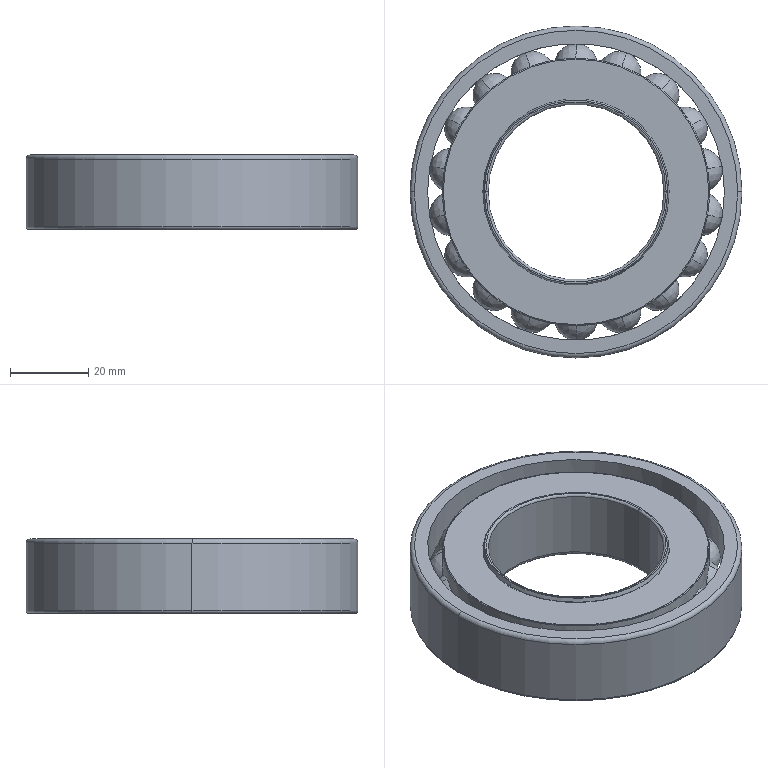Part | SolidWorks | features Revolution 5, Fillet 2, CirPattern 1, LockFeature 1, RefAxis 1 | 1 solid | 113 faces | box 85 x 85 x 19 mm | volume 41492 mm3 | plane 43 | sphere 36 | cylinder 16 | torus 12 | cone 6 | commonest cylinder face diameters 68 x4 45 x2 54 x2 67.4 x2 68.4 x2 76 x2